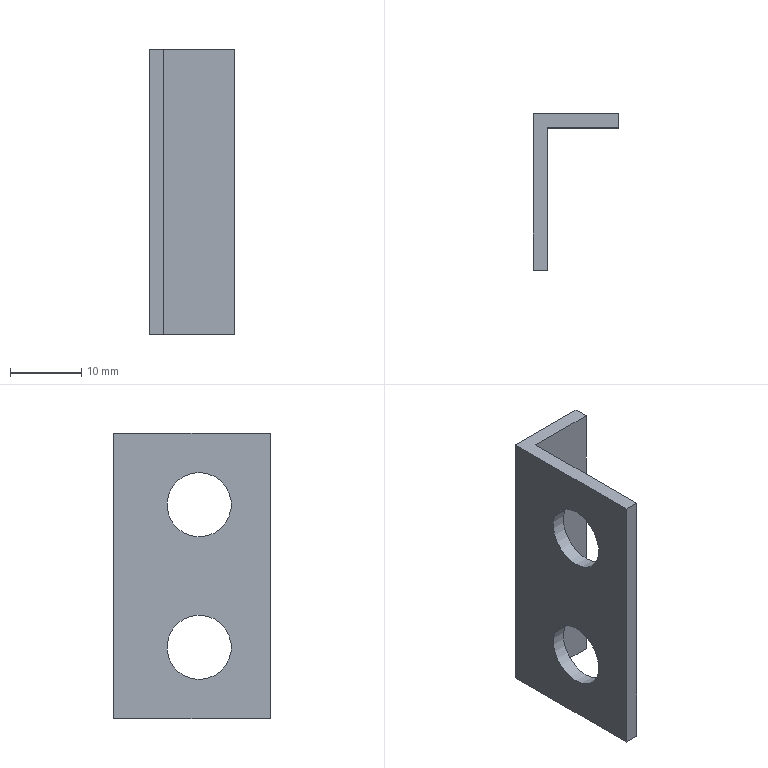Part | STEP file | lll_id4290_x_t | 1 solid | 10 faces | box 12 x 22 x 40 mm | volume 2306 mm3 | plane 8 | cylinder 2 | commonest cylinder face diameters 9 x2
STEP:
#1=CARTESIAN_POINT('',(3967.435,-40.,-118.));
#2=VERTEX_POINT('',#1);
#3=CARTESIAN_POINT('',(3969.435,-40.,-118.));
#4=VERTEX_POINT('',#3);
#5=CARTESIAN_POINT('',(3967.435,-40.,-118.));
#6=DIRECTION('',(1.,0.,0.));
#7=VECTOR('',#6,1.);
#8=LINE('',#5,#7);
#9=EDGE_CURVE('',#2,#4,#8,.T.);
#10=ORIENTED_EDGE('',*,*,#9,.F.);
#11=CARTESIAN_POINT('',(3967.435,-40.,-158.));
#12=VERTEX_POINT('',#11);
#13=CARTESIAN_POINT('',(3967.435,-40.,-155.));
#14=DIRECTION('',(0.,0.,1.));
#15=VECTOR('',#14,1.);
#16=LINE('',#13,#15);
#17=EDGE_CURVE('',#12,#2,#16,.T.);
#18=ORIENTED_EDGE('',*,*,#17,.F.);
#19=CARTESIAN_POINT('',(3969.435,-40.,-158.));
#20=VERTEX_POINT('',#19);
#21=CARTESIAN_POINT('',(3967.435,-40.,-158.));
#22=DIRECTION('',(1.,0.,0.));
#23=VECTOR('',#22,1.);
#24=LINE('',#21,#23);
#25=EDGE_CURVE('',#12,#20,#24,.T.);
#26=ORIENTED_EDGE('',*,*,#25,.T.);
#27=CARTESIAN_POINT('',(3969.435,-40.,-155.));
#28=DIRECTION('',(0.,0.,1.));
#29=VECTOR('',#28,1.);
#30=LINE('',#27,#29);
#31=EDGE_CURVE('',#20,#4,#30,.T.);
#32=ORIENTED_EDGE('',*,*,#31,.T.);
#33=EDGE_LOOP('',(#10,#18,#26,#32));
#34=FACE_OUTER_BOUND('',#33,.T.);
#35=CARTESIAN_POINT('',(3967.435,-40.,-155.));
#36=DIRECTION('',(0.,-1.,0.));
#37=DIRECTION('',(0.,0.,1.));
#38=AXIS2_PLACEMENT_3D('',#35,#36,#37);
#39=PLANE('',#38);
#40=ADVANCED_FACE('',(#34),#39,.T.);
#41=CARTESIAN_POINT('',(3967.435,-18.,-118.));
#42=VERTEX_POINT('',#41);
#43=CARTESIAN_POINT('',(3967.435,560.,-118.));
#44=DIRECTION('',(0.,-1.,0.));
#45=VECTOR('',#44,1.);
#46=LINE('',#43,#45);
#47=EDGE_CURVE('',#42,#2,#46,.T.);
#48=ORIENTED_EDGE('',*,*,#47,.T.);
#49=ORIENTED_EDGE('',*,*,#9,.T.);
#50=CARTESIAN_POINT('',(3969.435,-20.,-118.));
#51=VERTEX_POINT('',#50);
#52=CARTESIAN_POINT('',(3969.435,560.,-118.));
#53=DIRECTION('',(0.,1.,0.));
#54=VECTOR('',#53,1.);
#55=LINE('',#52,#54);
#56=EDGE_CURVE('',#4,#51,#55,.T.);
#57=ORIENTED_EDGE('',*,*,#56,.T.);
#58=CARTESIAN_POINT('',(3979.435,-20.,-118.));
#59=VERTEX_POINT('',#58);
#60=CARTESIAN_POINT('',(3968.435,-20.,-118.));
#61=DIRECTION('',(-1.,0.,0.));
#62=VECTOR('',#61,1.);
#63=LINE('',#60,#62);
#64=EDGE_CURVE('',#59,#51,#63,.T.);
#65=ORIENTED_EDGE('',*,*,#64,.F.);
#66=CARTESIAN_POINT('',(3979.435,-18.,-118.));
#67=VERTEX_POINT('',#66);
#68=CARTESIAN_POINT('',(3979.435,-20.,-118.));
#69=DIRECTION('',(0.,1.,0.));
#70=VECTOR('',#69,1.);
#71=LINE('',#68,#70);
#72=EDGE_CURVE('',#59,#67,#71,.T.);
#73=ORIENTED_EDGE('',*,*,#72,.T.);
#74=CARTESIAN_POINT('',(3968.435,-18.,-118.));
#75=DIRECTION('',(-1.,0.,0.));
#76=VECTOR('',#75,1.);
#77=LINE('',#74,#76);
#78=EDGE_CURVE('',#67,#42,#77,.T.);
#79=ORIENTED_EDGE('',*,*,#78,.T.);
#80=EDGE_LOOP('',(#48,#49,#57,#65,#73,#79));
#81=FACE_OUTER_BOUND('',#80,.T.);
#82=CARTESIAN_POINT('',(3968.435,-8.5,-118.));
#83=DIRECTION('',(0.,0.,-1.));
#84=DIRECTION('',(-1.,0.,0.));
#85=AXIS2_PLACEMENT_3D('',#82,#83,#84);
#86=PLANE('',#85);
#87=ADVANCED_FACE('',(#81),#86,.F.);
#88=CARTESIAN_POINT('',(3967.435,-30.,-132.5));
#89=VERTEX_POINT('',#88);
#90=CARTESIAN_POINT('',(3967.435,-30.,-128.));
#91=DIRECTION('',(-1.,0.,0.));
#92=DIRECTION('',(0.,0.,-1.));
#93=AXIS2_PLACEMENT_3D('',#90,#91,#92);
#94=CIRCLE('',#93,4.5);
#95=EDGE_CURVE('',#89,#89,#94,.T.);
#96=ORIENTED_EDGE('',*,*,#95,.F.);
#97=EDGE_LOOP('',(#96));
#98=FACE_BOUND('',#97,.T.);
#99=CARTESIAN_POINT('',(3967.435,-18.,-158.));
#100=VERTEX_POINT('',#99);
#101=CARTESIAN_POINT('',(3967.435,-18.,-128.));
#102=DIRECTION('',(0.,0.,1.));
#103=VECTOR('',#102,1.);
#104=LINE('',#101,#103);
#105=EDGE_CURVE('',#100,#42,#104,.T.);
#106=ORIENTED_EDGE('',*,*,#105,.F.);
#107=CARTESIAN_POINT('',(3967.435,560.,-158.));
#108=DIRECTION('',(0.,-1.,0.));
#109=VECTOR('',#108,1.);
#110=LINE('',#107,#109);
#111=EDGE_CURVE('',#100,#12,#110,.T.);
#112=ORIENTED_EDGE('',*,*,#111,.T.);
#113=ORIENTED_EDGE('',*,*,#17,.T.);
#114=ORIENTED_EDGE('',*,*,#47,.F.);
#115=EDGE_LOOP('',(#106,#112,#113,#114));
#116=FACE_BOUND('',#115,.T.);
#117=CARTESIAN_POINT('',(3967.435,-30.,-152.5));
#118=VERTEX_POINT('',#117);
#119=CARTESIAN_POINT('',(3967.435,-30.,-148.));
#120=DIRECTION('',(-1.,0.,0.));
#121=DIRECTION('',(0.,0.,-1.));
#122=AXIS2_PLACEMENT_3D('',#119,#120,#121);
#123=CIRCLE('',#122,4.5);
#124=EDGE_CURVE('',#118,#118,#123,.T.);
#125=ORIENTED_EDGE('',*,*,#124,.F.);
#126=EDGE_LOOP('',(#125));
#127=FACE_BOUND('',#126,.T.);
#128=CARTESIAN_POINT('',(3967.435,560.,-155.));
#129=DIRECTION('',(1.,0.,0.));
#130=DIRECTION('',(0.,0.,-1.));
#131=AXIS2_PLACEMENT_3D('',#128,#129,#130);
#132=PLANE('',#131);
#133=ADVANCED_FACE('',(#98,#116,#127),#132,.F.);
#134=CARTESIAN_POINT('',(3969.435,-30.,-123.5));
#135=VERTEX_POINT('',#134);
#136=CARTESIAN_POINT('',(3969.435,-30.,-128.));
#137=DIRECTION('',(1.,0.,0.));
#138=DIRECTION('',(0.,0.,1.));
#139=AXIS2_PLACEMENT_3D('',#136,#137,#138);
#140=CIRCLE('',#139,4.5);
#141=EDGE_CURVE('',#135,#135,#140,.T.);
#142=ORIENTED_EDGE('',*,*,#141,.F.);
#143=EDGE_LOOP('',(#142));
#144=FACE_BOUND('',#143,.T.);
#145=CARTESIAN_POINT('',(3969.435,-20.,-158.));
#146=VERTEX_POINT('',#145);
#147=CARTESIAN_POINT('',(3969.435,-20.,-155.));
#148=DIRECTION('',(0.,0.,-1.));
#149=VECTOR('',#148,1.);
#150=LINE('',#147,#149);
#151=EDGE_CURVE('',#51,#146,#150,.T.);
#152=ORIENTED_EDGE('',*,*,#151,.F.);
#153=ORIENTED_EDGE('',*,*,#56,.F.);
#154=ORIENTED_EDGE('',*,*,#31,.F.);
#155=CARTESIAN_POINT('',(3969.435,560.,-158.));
#156=DIRECTION('',(0.,-1.,0.));
#157=VECTOR('',#156,1.);
#158=LINE('',#155,#157);
#159=EDGE_CURVE('',#146,#20,#158,.T.);
#160=ORIENTED_EDGE('',*,*,#159,.F.);
#161=EDGE_LOOP('',(#152,#153,#154,#160));
#162=FACE_BOUND('',#161,.T.);
#163=CARTESIAN_POINT('',(3969.435,-30.,-143.5));
#164=VERTEX_POINT('',#163);
#165=CARTESIAN_POINT('',(3969.435,-30.,-148.));
#166=DIRECTION('',(1.,0.,0.));
#167=DIRECTION('',(0.,0.,1.));
#168=AXIS2_PLACEMENT_3D('',#165,#166,#167);
#169=CIRCLE('',#168,4.5);
#170=EDGE_CURVE('',#164,#164,#169,.T.);
#171=ORIENTED_EDGE('',*,*,#170,.F.);
#172=EDGE_LOOP('',(#171));
#173=FACE_BOUND('',#172,.T.);
#174=CARTESIAN_POINT('',(3969.435,560.,-155.));
#175=DIRECTION('',(1.,0.,0.));
#176=DIRECTION('',(0.,0.,-1.));
#177=AXIS2_PLACEMENT_3D('',#174,#175,#176);
#178=PLANE('',#177);
#179=ADVANCED_FACE('',(#144,#162,#173),#178,.T.);
#180=ORIENTED_EDGE('',*,*,#151,.T.);
#181=CARTESIAN_POINT('',(3979.435,-20.,-158.));
#182=VERTEX_POINT('',#181);
#183=CARTESIAN_POINT('',(3967.435,-20.,-158.));
#184=DIRECTION('',(-1.,0.,0.));
#185=VECTOR('',#184,1.);
#186=LINE('',#183,#185);
#187=EDGE_CURVE('',#182,#146,#186,.T.);
#188=ORIENTED_EDGE('',*,*,#187,.F.);
#189=CARTESIAN_POINT('',(3979.435,-20.,-128.));
#190=DIRECTION('',(0.,0.,-1.));
#191=VECTOR('',#190,1.);
#192=LINE('',#189,#191);
#193=EDGE_CURVE('',#59,#182,#192,.T.);
#194=ORIENTED_EDGE('',*,*,#193,.F.);
#195=ORIENTED_EDGE('',*,*,#64,.T.);
#196=EDGE_LOOP('',(#180,#188,#194,#195));
#197=FACE_OUTER_BOUND('',#196,.T.);
#198=CARTESIAN_POINT('',(3968.435,-20.,-128.));
#199=DIRECTION('',(0.,-1.,0.));
#200=DIRECTION('',(0.,0.,1.));
#201=AXIS2_PLACEMENT_3D('',#198,#199,#200);
#202=PLANE('',#201);
#203=ADVANCED_FACE('',(#197),#202,.T.);
#204=ORIENTED_EDGE('',*,*,#193,.T.);
#205=CARTESIAN_POINT('',(3979.435,-18.,-158.));
#206=VERTEX_POINT('',#205);
#207=CARTESIAN_POINT('',(3979.435,-20.,-158.));
#208=DIRECTION('',(0.,1.,0.));
#209=VECTOR('',#208,1.);
#210=LINE('',#207,#209);
#211=EDGE_CURVE('',#182,#206,#210,.T.);
#212=ORIENTED_EDGE('',*,*,#211,.T.);
#213=CARTESIAN_POINT('',(3979.435,-18.,-128.));
#214=DIRECTION('',(0.,0.,-1.));
#215=VECTOR('',#214,1.);
#216=LINE('',#213,#215);
#217=EDGE_CURVE('',#67,#206,#216,.T.);
#218=ORIENTED_EDGE('',*,*,#217,.F.);
#219=ORIENTED_EDGE('',*,*,#72,.F.);
#220=EDGE_LOOP('',(#204,#212,#218,#219));
#221=FACE_OUTER_BOUND('',#220,.T.);
#222=CARTESIAN_POINT('',(3979.435,-20.,-155.));
#223=DIRECTION('',(-1.,0.,0.));
#224=DIRECTION('',(0.,0.,1.));
#225=AXIS2_PLACEMENT_3D('',#222,#223,#224);
#226=PLANE('',#225);
#227=ADVANCED_FACE('',(#221),#226,.F.);
#228=ORIENTED_EDGE('',*,*,#217,.T.);
#229=CARTESIAN_POINT('',(3968.435,-18.,-158.));
#230=DIRECTION('',(-1.,0.,0.));
#231=VECTOR('',#230,1.);
#232=LINE('',#229,#231);
#233=EDGE_CURVE('',#206,#100,#232,.T.);
#234=ORIENTED_EDGE('',*,*,#233,.T.);
#235=ORIENTED_EDGE('',*,*,#105,.T.);
#236=ORIENTED_EDGE('',*,*,#78,.F.);
#237=EDGE_LOOP('',(#228,#234,#235,#236));
#238=FACE_OUTER_BOUND('',#237,.T.);
#239=CARTESIAN_POINT('',(3968.435,-18.,-128.));
#240=DIRECTION('',(0.,-1.,0.));
#241=DIRECTION('',(0.,0.,1.));
#242=AXIS2_PLACEMENT_3D('',#239,#240,#241);
#243=PLANE('',#242);
#244=ADVANCED_FACE('',(#238),#243,.F.);
#245=ORIENTED_EDGE('',*,*,#141,.T.);
#246=EDGE_LOOP('',(#245));
#247=FACE_BOUND('',#246,.T.);
#248=ORIENTED_EDGE('',*,*,#95,.T.);
#249=EDGE_LOOP('',(#248));
#250=FACE_BOUND('',#249,.T.);
#251=CARTESIAN_POINT('',(3969.435,-30.,-128.));
#252=DIRECTION('',(-1.,0.,0.));
#253=DIRECTION('',(0.,0.,1.));
#254=AXIS2_PLACEMENT_3D('',#251,#252,#253);
#255=CYLINDRICAL_SURFACE('',#254,4.5);
#256=ADVANCED_FACE('',(#247,#250),#255,.F.);
#257=ORIENTED_EDGE('',*,*,#159,.T.);
#258=ORIENTED_EDGE('',*,*,#25,.F.);
#259=ORIENTED_EDGE('',*,*,#111,.F.);
#260=ORIENTED_EDGE('',*,*,#233,.F.);
#261=ORIENTED_EDGE('',*,*,#211,.F.);
#262=ORIENTED_EDGE('',*,*,#187,.T.);
#263=EDGE_LOOP('',(#257,#258,#259,#260,#261,#262));
#264=FACE_OUTER_BOUND('',#263,.T.);
#265=CARTESIAN_POINT('',(3967.435,560.,-158.));
#266=DIRECTION('',(0.,0.,-1.));
#267=DIRECTION('',(0.,-1.,0.));
#268=AXIS2_PLACEMENT_3D('',#265,#266,#267);
#269=PLANE('',#268);
#270=ADVANCED_FACE('',(#264),#269,.T.);
#271=ORIENTED_EDGE('',*,*,#170,.T.);
#272=EDGE_LOOP('',(#271));
#273=FACE_BOUND('',#272,.T.);
#274=ORIENTED_EDGE('',*,*,#124,.T.);
#275=EDGE_LOOP('',(#274));
#276=FACE_BOUND('',#275,.T.);
#277=CARTESIAN_POINT('',(3969.435,-30.,-148.));
#278=DIRECTION('',(-1.,0.,0.));
#279=DIRECTION('',(0.,0.,1.));
#280=AXIS2_PLACEMENT_3D('',#277,#278,#279);
#281=CYLINDRICAL_SURFACE('',#280,4.5);
#282=ADVANCED_FACE('',(#273,#276),#281,.F.);
#283=CLOSED_SHELL('',(#40,#87,#133,#179,#203,#227,#244,#256,#270,#282));
#284=MANIFOLD_SOLID_BREP('',#283);
#285=(LENGTH_UNIT()NAMED_UNIT(*)SI_UNIT(.MILLI.,.METRE.));
#286=UNCERTAINTY_MEASURE_WITH_UNIT(LENGTH_MEASURE(0.00002),#285,'','');
#287=(NAMED_UNIT(*)PLANE_ANGLE_UNIT()SI_UNIT($,.RADIAN.));
#288=PLANE_ANGLE_MEASURE_WITH_UNIT(PLANE_ANGLE_MEASURE(0.01745),#287);
#289=DIMENSIONAL_EXPONENTS(0.,0.,0.,0.,0.,0.,0.);
#290=(CONVERSION_BASED_UNIT('DEGREE',#288)NAMED_UNIT(#289)PLANE_ANGLE_UNIT());
#291=(NAMED_UNIT(*)SI_UNIT($,.STERADIAN.)SOLID_ANGLE_UNIT());
#292=(GEOMETRIC_REPRESENTATION_CONTEXT(3)GLOBAL_UNCERTAINTY_ASSIGNED_CONTEXT((#286))GLOBAL_UNIT_ASSIGNED_CONTEXT((#285,#290,#291))REPRESENTATION_CONTEXT('',''));
#293=ADVANCED_BREP_SHAPE_REPRESENTATION('',(#284),#292);